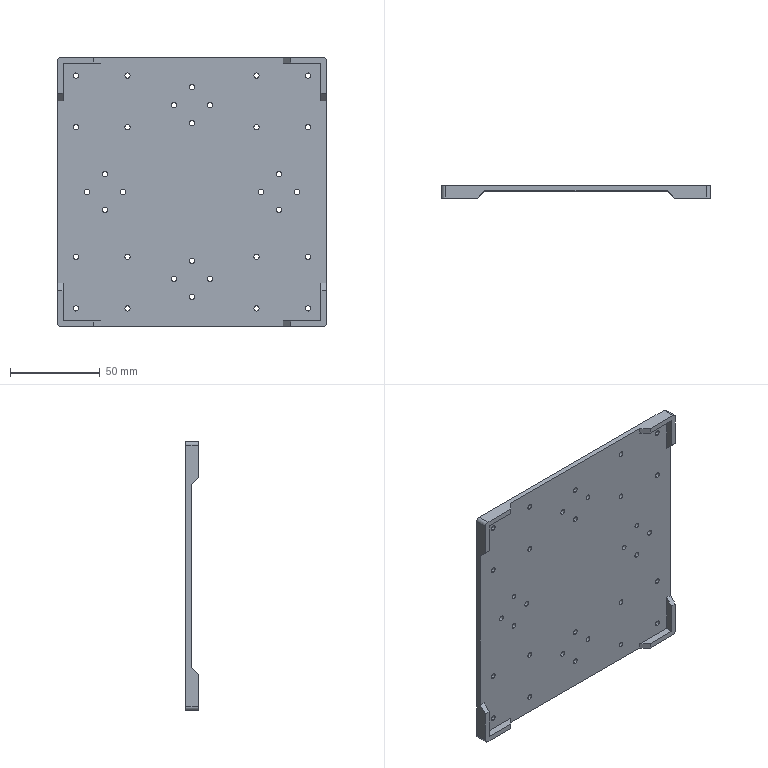Part | SolidWorks | features ICE 5, Extrusion 1, Fillet 1 | 1 solid | 94 faces | box 150 x 7 x 150 mm | volume 68792 mm3 | cylinder 68 | plane 26 | commonest cylinder face diameters 2.88 x32 3 x32 4 x4